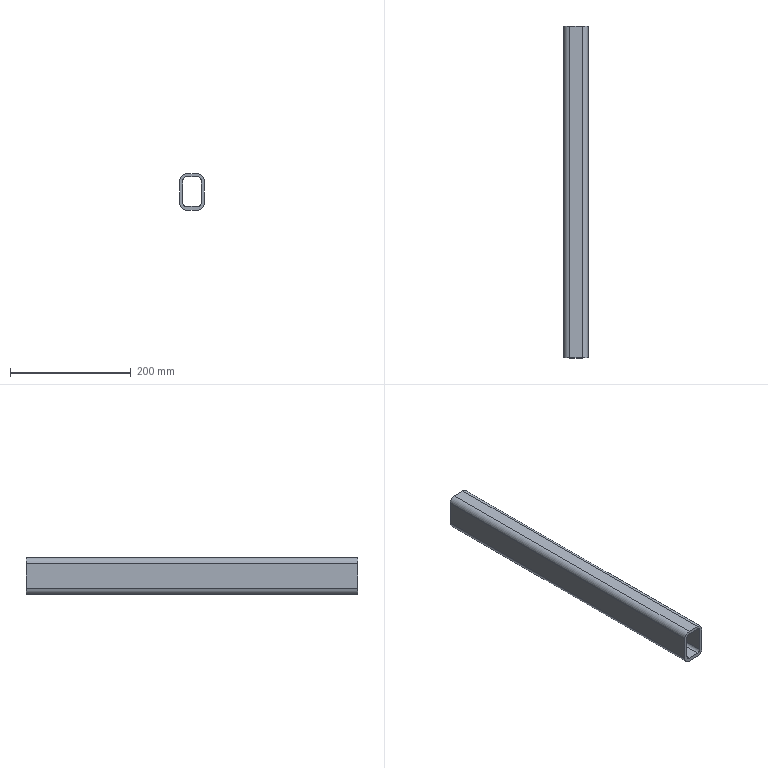Part | STEP file | frame longitudinal beam--000.001--20240926 | 1 solid | 18 faces | box 40 x 550 x 60 mm | volume 476091 mm3 | plane 10 | cylinder 8 | commonest cylinder face diameters 10 x4 20 x4
STEP:
#1=CARTESIAN_POINT('',(0.,0.,0.));
#2=DIRECTION('',(0.,0.,1.));
#3=DIRECTION('',(1.,0.,0.));
#4=AXIS2_PLACEMENT_3D('',#1,#2,#3);
#5=CARTESIAN_POINT('',(-30.,-840.,50.));
#6=VERTEX_POINT('',#5);
#7=CARTESIAN_POINT('',(-30.,-290.,50.));
#8=VERTEX_POINT('',#7);
#9=CARTESIAN_POINT('',(-30.,490.173,50.));
#10=DIRECTION('',(0.,1.,0.));
#11=VECTOR('',#10,1.);
#12=LINE('',#9,#11);
#13=CARTESIAN_POINT('',(-30.,490.173,40.));
#14=DIRECTION('',(0.,1.,0.));
#15=DIRECTION('',(0.,0.,-1.));
#16=AXIS2_PLACEMENT_3D('',#13,#14,#15);
#17=CYLINDRICAL_SURFACE('',#16,10.);
#18=CARTESIAN_POINT('',(3.142,0.));
#19=DIRECTION('',(0.,1.));
#20=VECTOR('',#19,1.);
#21=LINE('',#18,#20);
#22=(GEOMETRIC_REPRESENTATION_CONTEXT(2)PARAMETRIC_REPRESENTATION_CONTEXT()REPRESENTATION_CONTEXT('',''));
#23=DEFINITIONAL_REPRESENTATION('',(#21),#22);
#24=PCURVE('',#17,#23);
#25=CARTESIAN_POINT('',(-40.,490.173,50.));
#26=DIRECTION('',(0.,0.,-1.));
#27=DIRECTION('',(0.,-1.,0.));
#28=AXIS2_PLACEMENT_3D('',#25,#26,#27);
#29=PLANE('',#28);
#30=CARTESIAN_POINT('',(0.,-10.));
#31=DIRECTION('',(-1.,0.));
#32=VECTOR('',#31,1.);
#33=LINE('',#30,#32);
#34=(GEOMETRIC_REPRESENTATION_CONTEXT(2)PARAMETRIC_REPRESENTATION_CONTEXT()REPRESENTATION_CONTEXT('',''));
#35=DEFINITIONAL_REPRESENTATION('',(#33),#34);
#36=PCURVE('',#29,#35);
#37=SURFACE_CURVE('',#12,(#24,#36),.PCURVE_S1.);
#38=EDGE_CURVE('',#6,#8,#37,.T.);
#39=ORIENTED_EDGE('',*,*,#38,.T.);
#40=CARTESIAN_POINT('',(-40.,-290.,40.));
#41=VERTEX_POINT('',#40);
#42=CARTESIAN_POINT('',(-30.,-290.,40.));
#43=DIRECTION('',(0.,-1.,0.));
#44=DIRECTION('',(0.,0.,1.));
#45=AXIS2_PLACEMENT_3D('',#42,#43,#44);
#46=CIRCLE('',#45,10.);
#47=CARTESIAN_POINT('',(3.142,-780.173));
#48=DIRECTION('',(-1.,0.));
#49=VECTOR('',#48,1.);
#50=LINE('',#47,#49);
#51=(GEOMETRIC_REPRESENTATION_CONTEXT(2)PARAMETRIC_REPRESENTATION_CONTEXT()REPRESENTATION_CONTEXT('',''));
#52=DEFINITIONAL_REPRESENTATION('',(#50),#51);
#53=PCURVE('',#17,#52);
#54=CARTESIAN_POINT('',(-399.25,-290.,20.));
#55=DIRECTION('',(0.,1.,0.));
#56=DIRECTION('',(0.,0.,-1.));
#57=AXIS2_PLACEMENT_3D('',#54,#55,#56);
#58=PLANE('',#57);
#59=CARTESIAN_POINT('',(-30.,-369.25));
#60=CARTESIAN_POINT('',(-30.,-351.929));
#61=CARTESIAN_POINT('',(-15.,-360.59));
#62=CARTESIAN_POINT('',(0.,-369.25));
#63=CARTESIAN_POINT('',(-15.,-377.91));
#64=CARTESIAN_POINT('',(-30.,-386.571));
#65=CARTESIAN_POINT('',(-30.,-369.25));
#66=(BOUNDED_CURVE()B_SPLINE_CURVE(2,(#59,#60,#61,#62,#63,#64,#65),.UNSPECIFIED.,.T.,.F.)B_SPLINE_CURVE_WITH_KNOTS((1,2,2,2,2,1),(-2.094,0.,2.094,4.189,6.283,8.378),.UNSPECIFIED.)CURVE()GEOMETRIC_REPRESENTATION_ITEM()RATIONAL_B_SPLINE_CURVE((1.,0.5,1.,0.5,1.,0.5,1.))REPRESENTATION_ITEM(''));
#67=(GEOMETRIC_REPRESENTATION_CONTEXT(2)PARAMETRIC_REPRESENTATION_CONTEXT()REPRESENTATION_CONTEXT('',''));
#68=DEFINITIONAL_REPRESENTATION('',(#66),#67);
#69=PCURVE('',#58,#68);
#70=SURFACE_CURVE('',#46,(#53,#69),.PCURVE_S1.);
#71=EDGE_CURVE('',#8,#41,#70,.T.);
#72=ORIENTED_EDGE('',*,*,#71,.T.);
#73=CARTESIAN_POINT('',(-40.,-840.,40.));
#74=VERTEX_POINT('',#73);
#75=CARTESIAN_POINT('',(-40.,490.173,40.));
#76=DIRECTION('',(0.,-1.,0.));
#77=VECTOR('',#76,1.);
#78=LINE('',#75,#77);
#79=CARTESIAN_POINT('',(1.571,0.));
#80=DIRECTION('',(0.,-1.));
#81=VECTOR('',#80,1.);
#82=LINE('',#79,#81);
#83=(GEOMETRIC_REPRESENTATION_CONTEXT(2)PARAMETRIC_REPRESENTATION_CONTEXT()REPRESENTATION_CONTEXT('',''));
#84=DEFINITIONAL_REPRESENTATION('',(#82),#83);
#85=PCURVE('',#17,#84);
#86=CARTESIAN_POINT('',(-40.,490.173,10.));
#87=DIRECTION('',(1.,0.,0.));
#88=DIRECTION('',(0.,0.9613,-0.2756));
#89=AXIS2_PLACEMENT_3D('',#86,#87,#88);
#90=PLANE('',#89);
#91=CARTESIAN_POINT('',(-8.269,28.838));
#92=DIRECTION('',(-0.9613,-0.2756));
#93=VECTOR('',#92,1.);
#94=LINE('',#91,#93);
#95=(GEOMETRIC_REPRESENTATION_CONTEXT(2)PARAMETRIC_REPRESENTATION_CONTEXT()REPRESENTATION_CONTEXT('',''));
#96=DEFINITIONAL_REPRESENTATION('',(#94),#95);
#97=PCURVE('',#90,#96);
#98=SURFACE_CURVE('',#78,(#85,#97),.PCURVE_S1.);
#99=EDGE_CURVE('',#41,#74,#98,.T.);
#100=ORIENTED_EDGE('',*,*,#99,.T.);
#101=CARTESIAN_POINT('',(-30.,-840.,40.));
#102=DIRECTION('',(0.,-1.,0.));
#103=DIRECTION('',(0.,0.,1.));
#104=AXIS2_PLACEMENT_3D('',#101,#102,#103);
#105=CIRCLE('',#104,10.);
#106=CARTESIAN_POINT('',(3.142,-1330.173));
#107=DIRECTION('',(-1.,0.));
#108=VECTOR('',#107,1.);
#109=LINE('',#106,#108);
#110=(GEOMETRIC_REPRESENTATION_CONTEXT(2)PARAMETRIC_REPRESENTATION_CONTEXT()REPRESENTATION_CONTEXT('',''));
#111=DEFINITIONAL_REPRESENTATION('',(#109),#110);
#112=PCURVE('',#17,#111);
#113=CARTESIAN_POINT('',(-40.,-840.,-10.));
#114=DIRECTION('',(0.,1.,0.));
#115=DIRECTION('',(0.,0.,-1.));
#116=AXIS2_PLACEMENT_3D('',#113,#114,#115);
#117=PLANE('',#116);
#118=CARTESIAN_POINT('',(-60.,-10.));
#119=CARTESIAN_POINT('',(-60.,7.321));
#120=CARTESIAN_POINT('',(-45.,-1.34));
#121=CARTESIAN_POINT('',(-30.,-10.));
#122=CARTESIAN_POINT('',(-45.,-18.66));
#123=CARTESIAN_POINT('',(-60.,-27.321));
#124=CARTESIAN_POINT('',(-60.,-10.));
#125=(BOUNDED_CURVE()B_SPLINE_CURVE(2,(#118,#119,#120,#121,#122,#123,#124),.UNSPECIFIED.,.T.,.F.)B_SPLINE_CURVE_WITH_KNOTS((1,2,2,2,2,1),(-2.094,0.,2.094,4.189,6.283,8.378),.UNSPECIFIED.)CURVE()GEOMETRIC_REPRESENTATION_ITEM()RATIONAL_B_SPLINE_CURVE((1.,0.5,1.,0.5,1.,0.5,1.))REPRESENTATION_ITEM(''));
#126=(GEOMETRIC_REPRESENTATION_CONTEXT(2)PARAMETRIC_REPRESENTATION_CONTEXT()REPRESENTATION_CONTEXT('',''));
#127=DEFINITIONAL_REPRESENTATION('',(#125),#126);
#128=PCURVE('',#117,#127);
#129=SURFACE_CURVE('',#105,(#112,#128),.PCURVE_S1.);
#130=EDGE_CURVE('',#6,#74,#129,.T.);
#131=ORIENTED_EDGE('',*,*,#130,.F.);
#132=EDGE_LOOP('',(#39,#72,#100,#131));
#133=FACE_BOUND('',#132,.T.);
#134=ADVANCED_FACE('',(#133),#17,.T.);
#135=CARTESIAN_POINT('',(-40.,-840.,0.));
#136=VERTEX_POINT('',#135);
#137=CARTESIAN_POINT('',(-40.,-290.,0.));
#138=VERTEX_POINT('',#137);
#139=CARTESIAN_POINT('',(-40.,1110.173,0.));
#140=DIRECTION('',(0.,1.,0.));
#141=VECTOR('',#140,1.);
#142=LINE('',#139,#141);
#143=CARTESIAN_POINT('',(-30.,1110.173,0.));
#144=DIRECTION('',(0.,1.,0.));
#145=DIRECTION('',(0.,0.,-1.));
#146=AXIS2_PLACEMENT_3D('',#143,#144,#145);
#147=CYLINDRICAL_SURFACE('',#146,10.);
#148=CARTESIAN_POINT('',(1.571,0.));
#149=DIRECTION('',(0.,1.));
#150=VECTOR('',#149,1.);
#151=LINE('',#148,#150);
#152=(GEOMETRIC_REPRESENTATION_CONTEXT(2)PARAMETRIC_REPRESENTATION_CONTEXT()REPRESENTATION_CONTEXT('',''));
#153=DEFINITIONAL_REPRESENTATION('',(#151),#152);
#154=PCURVE('',#147,#153);
#155=CARTESIAN_POINT('',(598.739,161.283));
#156=DIRECTION('',(0.9613,0.2756));
#157=VECTOR('',#156,1.);
#158=LINE('',#155,#157);
#159=(GEOMETRIC_REPRESENTATION_CONTEXT(2)PARAMETRIC_REPRESENTATION_CONTEXT()REPRESENTATION_CONTEXT('',''));
#160=DEFINITIONAL_REPRESENTATION('',(#158),#159);
#161=PCURVE('',#90,#160);
#162=SURFACE_CURVE('',#142,(#154,#161),.PCURVE_S1.);
#163=EDGE_CURVE('',#136,#138,#162,.T.);
#164=ORIENTED_EDGE('',*,*,#163,.T.);
#165=CARTESIAN_POINT('',(-30.,-290.,-10.));
#166=VERTEX_POINT('',#165);
#167=CARTESIAN_POINT('',(-30.,-290.,0.));
#168=DIRECTION('',(0.,-1.,0.));
#169=DIRECTION('',(0.,0.,1.));
#170=AXIS2_PLACEMENT_3D('',#167,#168,#169);
#171=CIRCLE('',#170,10.);
#172=CARTESIAN_POINT('',(3.142,-1400.173));
#173=DIRECTION('',(-1.,0.));
#174=VECTOR('',#173,1.);
#175=LINE('',#172,#174);
#176=(GEOMETRIC_REPRESENTATION_CONTEXT(2)PARAMETRIC_REPRESENTATION_CONTEXT()REPRESENTATION_CONTEXT('',''));
#177=DEFINITIONAL_REPRESENTATION('',(#175),#176);
#178=PCURVE('',#147,#177);
#179=CARTESIAN_POINT('',(10.,-369.25));
#180=CARTESIAN_POINT('',(10.,-351.929));
#181=CARTESIAN_POINT('',(25.,-360.59));
#182=CARTESIAN_POINT('',(40.,-369.25));
#183=CARTESIAN_POINT('',(25.,-377.91));
#184=CARTESIAN_POINT('',(10.,-386.571));
#185=CARTESIAN_POINT('',(10.,-369.25));
#186=(BOUNDED_CURVE()B_SPLINE_CURVE(2,(#179,#180,#181,#182,#183,#184,#185),.UNSPECIFIED.,.T.,.F.)B_SPLINE_CURVE_WITH_KNOTS((1,2,2,2,2,1),(-2.094,0.,2.094,4.189,6.283,8.378),.UNSPECIFIED.)CURVE()GEOMETRIC_REPRESENTATION_ITEM()RATIONAL_B_SPLINE_CURVE((1.,0.5,1.,0.5,1.,0.5,1.))REPRESENTATION_ITEM(''));
#187=(GEOMETRIC_REPRESENTATION_CONTEXT(2)PARAMETRIC_REPRESENTATION_CONTEXT()REPRESENTATION_CONTEXT('',''));
#188=DEFINITIONAL_REPRESENTATION('',(#186),#187);
#189=PCURVE('',#58,#188);
#190=SURFACE_CURVE('',#171,(#178,#189),.PCURVE_S1.);
#191=EDGE_CURVE('',#138,#166,#190,.T.);
#192=ORIENTED_EDGE('',*,*,#191,.T.);
#193=CARTESIAN_POINT('',(-30.,-840.,-10.));
#194=VERTEX_POINT('',#193);
#195=CARTESIAN_POINT('',(-30.,1110.173,-10.));
#196=DIRECTION('',(0.,-1.,0.));
#197=VECTOR('',#196,1.);
#198=LINE('',#195,#197);
#199=CARTESIAN_POINT('',(0.,0.));
#200=DIRECTION('',(0.,-1.));
#201=VECTOR('',#200,1.);
#202=LINE('',#199,#201);
#203=(GEOMETRIC_REPRESENTATION_CONTEXT(2)PARAMETRIC_REPRESENTATION_CONTEXT()REPRESENTATION_CONTEXT('',''));
#204=DEFINITIONAL_REPRESENTATION('',(#202),#203);
#205=PCURVE('',#147,#204);
#206=CARTESIAN_POINT('',(0.,1110.173,-10.));
#207=DIRECTION('',(0.,0.,1.));
#208=DIRECTION('',(0.,1.,0.));
#209=AXIS2_PLACEMENT_3D('',#206,#207,#208);
#210=PLANE('',#209);
#211=CARTESIAN_POINT('',(0.,30.));
#212=DIRECTION('',(-1.,0.));
#213=VECTOR('',#212,1.);
#214=LINE('',#211,#213);
#215=(GEOMETRIC_REPRESENTATION_CONTEXT(2)PARAMETRIC_REPRESENTATION_CONTEXT()REPRESENTATION_CONTEXT('',''));
#216=DEFINITIONAL_REPRESENTATION('',(#214),#215);
#217=PCURVE('',#210,#216);
#218=SURFACE_CURVE('',#198,(#205,#217),.PCURVE_S1.);
#219=EDGE_CURVE('',#166,#194,#218,.T.);
#220=ORIENTED_EDGE('',*,*,#219,.T.);
#221=CARTESIAN_POINT('',(-30.,-840.,0.));
#222=DIRECTION('',(0.,-1.,0.));
#223=DIRECTION('',(0.,0.,1.));
#224=AXIS2_PLACEMENT_3D('',#221,#222,#223);
#225=CIRCLE('',#224,10.);
#226=CARTESIAN_POINT('',(3.142,-1950.173));
#227=DIRECTION('',(-1.,0.));
#228=VECTOR('',#227,1.);
#229=LINE('',#226,#228);
#230=(GEOMETRIC_REPRESENTATION_CONTEXT(2)PARAMETRIC_REPRESENTATION_CONTEXT()REPRESENTATION_CONTEXT('',''));
#231=DEFINITIONAL_REPRESENTATION('',(#229),#230);
#232=PCURVE('',#147,#231);
#233=CARTESIAN_POINT('',(-20.,-10.));
#234=CARTESIAN_POINT('',(-20.,7.321));
#235=CARTESIAN_POINT('',(-5.,-1.34));
#236=CARTESIAN_POINT('',(10.,-10.));
#237=CARTESIAN_POINT('',(-5.,-18.66));
#238=CARTESIAN_POINT('',(-20.,-27.321));
#239=CARTESIAN_POINT('',(-20.,-10.));
#240=(BOUNDED_CURVE()B_SPLINE_CURVE(2,(#233,#234,#235,#236,#237,#238,#239),.UNSPECIFIED.,.T.,.F.)B_SPLINE_CURVE_WITH_KNOTS((1,2,2,2,2,1),(-2.094,0.,2.094,4.189,6.283,8.378),.UNSPECIFIED.)CURVE()GEOMETRIC_REPRESENTATION_ITEM()RATIONAL_B_SPLINE_CURVE((1.,0.5,1.,0.5,1.,0.5,1.))REPRESENTATION_ITEM(''));
#241=(GEOMETRIC_REPRESENTATION_CONTEXT(2)PARAMETRIC_REPRESENTATION_CONTEXT()REPRESENTATION_CONTEXT('',''));
#242=DEFINITIONAL_REPRESENTATION('',(#240),#241);
#243=PCURVE('',#117,#242);
#244=SURFACE_CURVE('',#225,(#232,#243),.PCURVE_S1.);
#245=EDGE_CURVE('',#136,#194,#244,.T.);
#246=ORIENTED_EDGE('',*,*,#245,.F.);
#247=EDGE_LOOP('',(#164,#192,#220,#246));
#248=FACE_BOUND('',#247,.T.);
#249=ADVANCED_FACE('',(#248),#147,.T.);
#250=CARTESIAN_POINT('',(-40.,-290.,10.));
#251=DIRECTION('',(0.,0.,1.));
#252=VECTOR('',#251,1.);
#253=LINE('',#250,#252);
#254=CARTESIAN_POINT('',(-749.951,-215.045));
#255=DIRECTION('',(-0.2756,0.9613));
#256=VECTOR('',#255,1.);
#257=LINE('',#254,#256);
#258=(GEOMETRIC_REPRESENTATION_CONTEXT(2)PARAMETRIC_REPRESENTATION_CONTEXT()REPRESENTATION_CONTEXT('',''));
#259=DEFINITIONAL_REPRESENTATION('',(#257),#258);
#260=PCURVE('',#90,#259);
#261=CARTESIAN_POINT('',(10.,-359.25));
#262=DIRECTION('',(-1.,0.));
#263=VECTOR('',#262,1.);
#264=LINE('',#261,#263);
#265=(GEOMETRIC_REPRESENTATION_CONTEXT(2)PARAMETRIC_REPRESENTATION_CONTEXT()REPRESENTATION_CONTEXT('',''));
#266=DEFINITIONAL_REPRESENTATION('',(#264),#265);
#267=PCURVE('',#58,#266);
#268=SURFACE_CURVE('',#253,(#260,#267),.PCURVE_S1.);
#269=EDGE_CURVE('',#138,#41,#268,.T.);
#270=ORIENTED_EDGE('',*,*,#269,.F.);
#271=ORIENTED_EDGE('',*,*,#163,.F.);
#272=CARTESIAN_POINT('',(-40.,-840.,10.));
#273=DIRECTION('',(0.,0.,1.));
#274=VECTOR('',#273,1.);
#275=LINE('',#272,#274);
#276=CARTESIAN_POINT('',(-1278.645,-366.645));
#277=DIRECTION('',(-0.2756,0.9613));
#278=VECTOR('',#277,1.);
#279=LINE('',#276,#278);
#280=(GEOMETRIC_REPRESENTATION_CONTEXT(2)PARAMETRIC_REPRESENTATION_CONTEXT()REPRESENTATION_CONTEXT('',''));
#281=DEFINITIONAL_REPRESENTATION('',(#279),#280);
#282=PCURVE('',#90,#281);
#283=CARTESIAN_POINT('',(-20.,0.));
#284=DIRECTION('',(-1.,0.));
#285=VECTOR('',#284,1.);
#286=LINE('',#283,#285);
#287=(GEOMETRIC_REPRESENTATION_CONTEXT(2)PARAMETRIC_REPRESENTATION_CONTEXT()REPRESENTATION_CONTEXT('',''));
#288=DEFINITIONAL_REPRESENTATION('',(#286),#287);
#289=PCURVE('',#117,#288);
#290=SURFACE_CURVE('',#275,(#282,#289),.PCURVE_S1.);
#291=EDGE_CURVE('',#136,#74,#290,.T.);
#292=ORIENTED_EDGE('',*,*,#291,.T.);
#293=ORIENTED_EDGE('',*,*,#99,.F.);
#294=EDGE_LOOP('',(#270,#271,#292,#293));
#295=FACE_BOUND('',#294,.T.);
#296=ADVANCED_FACE('',(#295),#90,.F.);
#297=CARTESIAN_POINT('',(-10.,-840.,-10.));
#298=VERTEX_POINT('',#297);
#299=CARTESIAN_POINT('',(-10.,-290.,-10.));
#300=VERTEX_POINT('',#299);
#301=CARTESIAN_POINT('',(-10.,490.173,-10.));
#302=DIRECTION('',(0.,1.,0.));
#303=VECTOR('',#302,1.);
#304=LINE('',#301,#303);
#305=CARTESIAN_POINT('',(-10.,490.173,0.));
#306=DIRECTION('',(0.,1.,0.));
#307=DIRECTION('',(0.,0.,-1.));
#308=AXIS2_PLACEMENT_3D('',#305,#306,#307);
#309=CYLINDRICAL_SURFACE('',#308,10.);
#310=CARTESIAN_POINT('',(6.283,0.));
#311=DIRECTION('',(0.,1.));
#312=VECTOR('',#311,1.);
#313=LINE('',#310,#312);
#314=(GEOMETRIC_REPRESENTATION_CONTEXT(2)PARAMETRIC_REPRESENTATION_CONTEXT()REPRESENTATION_CONTEXT('',''));
#315=DEFINITIONAL_REPRESENTATION('',(#313),#314);
#316=PCURVE('',#309,#315);
#317=CARTESIAN_POINT('',(-620.,10.));
#318=DIRECTION('',(1.,0.));
#319=VECTOR('',#318,1.);
#320=LINE('',#317,#319);
#321=(GEOMETRIC_REPRESENTATION_CONTEXT(2)PARAMETRIC_REPRESENTATION_CONTEXT()REPRESENTATION_CONTEXT('',''));
#322=DEFINITIONAL_REPRESENTATION('',(#320),#321);
#323=PCURVE('',#210,#322);
#324=SURFACE_CURVE('',#304,(#316,#323),.PCURVE_S1.);
#325=EDGE_CURVE('',#298,#300,#324,.T.);
#326=ORIENTED_EDGE('',*,*,#325,.T.);
#327=CARTESIAN_POINT('',(0.,-290.,0.));
#328=VERTEX_POINT('',#327);
#329=CARTESIAN_POINT('',(-10.,-290.,0.));
#330=DIRECTION('',(0.,-1.,0.));
#331=DIRECTION('',(0.,0.,1.));
#332=AXIS2_PLACEMENT_3D('',#329,#330,#331);
#333=CIRCLE('',#332,10.);
#334=CARTESIAN_POINT('',(9.425,-780.173));
#335=DIRECTION('',(-1.,0.));
#336=VECTOR('',#335,1.);
#337=LINE('',#334,#336);
#338=(GEOMETRIC_REPRESENTATION_CONTEXT(2)PARAMETRIC_REPRESENTATION_CONTEXT()REPRESENTATION_CONTEXT('',''));
#339=DEFINITIONAL_REPRESENTATION('',(#337),#338);
#340=PCURVE('',#309,#339);
#341=CARTESIAN_POINT('',(10.,-389.25));
#342=CARTESIAN_POINT('',(10.,-371.929));
#343=CARTESIAN_POINT('',(25.,-380.59));
#344=CARTESIAN_POINT('',(40.,-389.25));
#345=CARTESIAN_POINT('',(25.,-397.91));
#346=CARTESIAN_POINT('',(10.,-406.571));
#347=CARTESIAN_POINT('',(10.,-389.25));
#348=(BOUNDED_CURVE()B_SPLINE_CURVE(2,(#341,#342,#343,#344,#345,#346,#347),.UNSPECIFIED.,.T.,.F.)B_SPLINE_CURVE_WITH_KNOTS((1,2,2,2,2,1),(-2.094,0.,2.094,4.189,6.283,8.378),.UNSPECIFIED.)CURVE()GEOMETRIC_REPRESENTATION_ITEM()RATIONAL_B_SPLINE_CURVE((1.,0.5,1.,0.5,1.,0.5,1.))REPRESENTATION_ITEM(''));
#349=(GEOMETRIC_REPRESENTATION_CONTEXT(2)PARAMETRIC_REPRESENTATION_CONTEXT()REPRESENTATION_CONTEXT('',''));
#350=DEFINITIONAL_REPRESENTATION('',(#348),#349);
#351=PCURVE('',#58,#350);
#352=SURFACE_CURVE('',#333,(#340,#351),.PCURVE_S1.);
#353=EDGE_CURVE('',#300,#328,#352,.T.);
#354=ORIENTED_EDGE('',*,*,#353,.T.);
#355=CARTESIAN_POINT('',(0.,-840.,0.));
#356=VERTEX_POINT('',#355);
#357=CARTESIAN_POINT('',(0.,490.173,0.));
#358=DIRECTION('',(0.,-1.,0.));
#359=VECTOR('',#358,1.);
#360=LINE('',#357,#359);
#361=CARTESIAN_POINT('',(4.712,0.));
#362=DIRECTION('',(0.,-1.));
#363=VECTOR('',#362,1.);
#364=LINE('',#361,#363);
#365=(GEOMETRIC_REPRESENTATION_CONTEXT(2)PARAMETRIC_REPRESENTATION_CONTEXT()REPRESENTATION_CONTEXT('',''));
#366=DEFINITIONAL_REPRESENTATION('',(#364),#365);
#367=PCURVE('',#309,#366);
#368=CARTESIAN_POINT('',(0.,490.173,50.));
#369=DIRECTION('',(-1.,0.,0.));
#370=DIRECTION('',(0.,-0.9613,0.2756));
#371=AXIS2_PLACEMENT_3D('',#368,#369,#370);
#372=PLANE('',#371);
#373=CARTESIAN_POINT('',(-13.782,-48.063));
#374=DIRECTION('',(0.9613,-0.2756));
#375=VECTOR('',#374,1.);
#376=LINE('',#373,#375);
#377=(GEOMETRIC_REPRESENTATION_CONTEXT(2)PARAMETRIC_REPRESENTATION_CONTEXT()REPRESENTATION_CONTEXT('',''));
#378=DEFINITIONAL_REPRESENTATION('',(#376),#377);
#379=PCURVE('',#372,#378);
#380=SURFACE_CURVE('',#360,(#367,#379),.PCURVE_S1.);
#381=EDGE_CURVE('',#328,#356,#380,.T.);
#382=ORIENTED_EDGE('',*,*,#381,.T.);
#383=CARTESIAN_POINT('',(-10.,-840.,0.));
#384=DIRECTION('',(0.,1.,0.));
#385=DIRECTION('',(0.,0.,1.));
#386=AXIS2_PLACEMENT_3D('',#383,#384,#385);
#387=CIRCLE('',#386,10.);
#388=CARTESIAN_POINT('',(3.142,-1330.173));
#389=DIRECTION('',(1.,0.));
#390=VECTOR('',#389,1.);
#391=LINE('',#388,#390);
#392=(GEOMETRIC_REPRESENTATION_CONTEXT(2)PARAMETRIC_REPRESENTATION_CONTEXT()REPRESENTATION_CONTEXT('',''));
#393=DEFINITIONAL_REPRESENTATION('',(#391),#392);
#394=PCURVE('',#309,#393);
#395=CARTESIAN_POINT('',(-10.,-30.));
#396=DIRECTION('',(-1.,0.));
#397=AXIS2_PLACEMENT_2D('',#395,#396);
#398=CIRCLE('',#397,10.);
#399=(GEOMETRIC_REPRESENTATION_CONTEXT(2)PARAMETRIC_REPRESENTATION_CONTEXT()REPRESENTATION_CONTEXT('',''));
#400=DEFINITIONAL_REPRESENTATION('',(#398),#399);
#401=PCURVE('',#117,#400);
#402=SURFACE_CURVE('',#387,(#394,#401),.PCURVE_S1.);
#403=EDGE_CURVE('',#356,#298,#402,.T.);
#404=ORIENTED_EDGE('',*,*,#403,.T.);
#405=EDGE_LOOP('',(#326,#354,#382,#404));
#406=FACE_BOUND('',#405,.T.);
#407=ADVANCED_FACE('',(#406),#309,.T.);
#408=CARTESIAN_POINT('',(0.,-290.,-10.));
#409=DIRECTION('',(-1.,0.,0.));
#410=VECTOR('',#409,1.);
#411=LINE('',#408,#410);
#412=CARTESIAN_POINT('',(-1400.173,0.));
#413=DIRECTION('',(0.,1.));
#414=VECTOR('',#413,1.);
#415=LINE('',#412,#414);
#416=(GEOMETRIC_REPRESENTATION_CONTEXT(2)PARAMETRIC_REPRESENTATION_CONTEXT()REPRESENTATION_CONTEXT('',''));
#417=DEFINITIONAL_REPRESENTATION('',(#415),#416);
#418=PCURVE('',#210,#417);
#419=CARTESIAN_POINT('',(30.,-399.25));
#420=DIRECTION('',(0.,1.));
#421=VECTOR('',#420,1.);
#422=LINE('',#419,#421);
#423=(GEOMETRIC_REPRESENTATION_CONTEXT(2)PARAMETRIC_REPRESENTATION_CONTEXT()REPRESENTATION_CONTEXT('',''));
#424=DEFINITIONAL_REPRESENTATION('',(#422),#423);
#425=PCURVE('',#58,#424);
#426=SURFACE_CURVE('',#411,(#418,#425),.PCURVE_S1.);
#427=EDGE_CURVE('',#300,#166,#426,.T.);
#428=ORIENTED_EDGE('',*,*,#427,.F.);
#429=ORIENTED_EDGE('',*,*,#325,.F.);
#430=CARTESIAN_POINT('',(-40.,-840.,-10.));
#431=DIRECTION('',(1.,0.,0.));
#432=VECTOR('',#431,1.);
#433=LINE('',#430,#432);
#434=CARTESIAN_POINT('',(-1950.173,40.));
#435=DIRECTION('',(0.,-1.));
#436=VECTOR('',#435,1.);
#437=LINE('',#434,#436);
#438=(GEOMETRIC_REPRESENTATION_CONTEXT(2)PARAMETRIC_REPRESENTATION_CONTEXT()REPRESENTATION_CONTEXT('',''));
#439=DEFINITIONAL_REPRESENTATION('',(#437),#438);
#440=PCURVE('',#210,#439);
#441=CARTESIAN_POINT('',(0.,0.));
#442=DIRECTION('',(0.,-1.));
#443=VECTOR('',#442,1.);
#444=LINE('',#441,#443);
#445=(GEOMETRIC_REPRESENTATION_CONTEXT(2)PARAMETRIC_REPRESENTATION_CONTEXT()REPRESENTATION_CONTEXT('',''));
#446=DEFINITIONAL_REPRESENTATION('',(#444),#445);
#447=PCURVE('',#117,#446);
#448=SURFACE_CURVE('',#433,(#440,#447),.PCURVE_S1.);
#449=EDGE_CURVE('',#194,#298,#448,.T.);
#450=ORIENTED_EDGE('',*,*,#449,.F.);
#451=ORIENTED_EDGE('',*,*,#219,.F.);
#452=EDGE_LOOP('',(#428,#429,#450,#451));
#453=FACE_BOUND('',#452,.T.);
#454=ADVANCED_FACE('',(#453),#210,.F.);
#455=CARTESIAN_POINT('',(0.,-840.,40.));
#456=VERTEX_POINT('',#455);
#457=CARTESIAN_POINT('',(0.,-290.,40.));
#458=VERTEX_POINT('',#457);
#459=CARTESIAN_POINT('',(0.,490.173,40.));
#460=DIRECTION('',(0.,1.,0.));
#461=VECTOR('',#460,1.);
#462=LINE('',#459,#461);
#463=CARTESIAN_POINT('',(-10.,490.173,40.));
#464=DIRECTION('',(0.,1.,0.));
#465=DIRECTION('',(0.,0.,-1.));
#466=AXIS2_PLACEMENT_3D('',#463,#464,#465);
#467=CYLINDRICAL_SURFACE('',#466,10.);
#468=CARTESIAN_POINT('',(4.712,0.));
#469=DIRECTION('',(0.,1.));
#470=VECTOR('',#469,1.);
#471=LINE('',#468,#470);
#472=(GEOMETRIC_REPRESENTATION_CONTEXT(2)PARAMETRIC_REPRESENTATION_CONTEXT()REPRESENTATION_CONTEXT('',''));
#473=DEFINITIONAL_REPRESENTATION('',(#471),#472);
#474=PCURVE('',#467,#473);
#475=CARTESIAN_POINT('',(-2.756,-9.613));
#476=DIRECTION('',(-0.9613,0.2756));
#477=VECTOR('',#476,1.);
#478=LINE('',#475,#477);
#479=(GEOMETRIC_REPRESENTATION_CONTEXT(2)PARAMETRIC_REPRESENTATION_CONTEXT()REPRESENTATION_CONTEXT('',''));
#480=DEFINITIONAL_REPRESENTATION('',(#478),#479);
#481=PCURVE('',#372,#480);
#482=SURFACE_CURVE('',#462,(#474,#481),.PCURVE_S1.);
#483=EDGE_CURVE('',#456,#458,#482,.T.);
#484=ORIENTED_EDGE('',*,*,#483,.T.);
#485=CARTESIAN_POINT('',(-10.,-290.,50.));
#486=VERTEX_POINT('',#485);
#487=CARTESIAN_POINT('',(-10.,-290.,40.));
#488=DIRECTION('',(0.,-1.,0.));
#489=DIRECTION('',(0.,0.,1.));
#490=AXIS2_PLACEMENT_3D('',#487,#488,#489);
#491=CIRCLE('',#490,10.);
#492=CARTESIAN_POINT('',(9.425,-780.173));
#493=DIRECTION('',(-1.,0.));
#494=VECTOR('',#493,1.);
#495=LINE('',#492,#494);
#496=(GEOMETRIC_REPRESENTATION_CONTEXT(2)PARAMETRIC_REPRESENTATION_CONTEXT()REPRESENTATION_CONTEXT('',''));
#497=DEFINITIONAL_REPRESENTATION('',(#495),#496);
#498=PCURVE('',#467,#497);
#499=CARTESIAN_POINT('',(-30.,-389.25));
#500=CARTESIAN_POINT('',(-30.,-371.929));
#501=CARTESIAN_POINT('',(-15.,-380.59));
#502=CARTESIAN_POINT('',(0.,-389.25));
#503=CARTESIAN_POINT('',(-15.,-397.91));
#504=CARTESIAN_POINT('',(-30.,-406.571));
#505=CARTESIAN_POINT('',(-30.,-389.25));
#506=(BOUNDED_CURVE()B_SPLINE_CURVE(2,(#499,#500,#501,#502,#503,#504,#505),.UNSPECIFIED.,.T.,.F.)B_SPLINE_CURVE_WITH_KNOTS((1,2,2,2,2,1),(-2.094,0.,2.094,4.189,6.283,8.378),.UNSPECIFIED.)CURVE()GEOMETRIC_REPRESENTATION_ITEM()RATIONAL_B_SPLINE_CURVE((1.,0.5,1.,0.5,1.,0.5,1.))REPRESENTATION_ITEM(''));
#507=(GEOMETRIC_REPRESENTATION_CONTEXT(2)PARAMETRIC_REPRESENTATION_CONTEXT()REPRESENTATION_CONTEXT('',''));
#508=DEFINITIONAL_REPRESENTATION('',(#506),#507);
#509=PCURVE('',#58,#508);
#510=SURFACE_CURVE('',#491,(#498,#509),.PCURVE_S1.);
#511=EDGE_CURVE('',#458,#486,#510,.T.);
#512=ORIENTED_EDGE('',*,*,#511,.T.);
#513=CARTESIAN_POINT('',(-10.,-840.,50.));
#514=VERTEX_POINT('',#513);
#515=CARTESIAN_POINT('',(-10.,490.173,50.));
#516=DIRECTION('',(0.,-1.,0.));
#517=VECTOR('',#516,1.);
#518=LINE('',#515,#517);
#519=CARTESIAN_POINT('',(3.142,0.));
#520=DIRECTION('',(0.,-1.));
#521=VECTOR('',#520,1.);
#522=LINE('',#519,#521);
#523=(GEOMETRIC_REPRESENTATION_CONTEXT(2)PARAMETRIC_REPRESENTATION_CONTEXT()REPRESENTATION_CONTEXT('',''));
#524=DEFINITIONAL_REPRESENTATION('',(#522),#523);
#525=PCURVE('',#467,#524);
#526=CARTESIAN_POINT('',(0.,-30.));
#527=DIRECTION('',(1.,0.));
#528=VECTOR('',#527,1.);
#529=LINE('',#526,#528);
#530=(GEOMETRIC_REPRESENTATION_CONTEXT(2)PARAMETRIC_REPRESENTATION_CONTEXT()REPRESENTATION_CONTEXT('',''));
#531=DEFINITIONAL_REPRESENTATION('',(#529),#530);
#532=PCURVE('',#29,#531);
#533=SURFACE_CURVE('',#518,(#525,#532),.PCURVE_S1.);
#534=EDGE_CURVE('',#486,#514,#533,.T.);
#535=ORIENTED_EDGE('',*,*,#534,.T.);
#536=CARTESIAN_POINT('',(-10.,-840.,40.));
#537=DIRECTION('',(0.,-1.,0.));
#538=DIRECTION('',(0.,0.,1.));
#539=AXIS2_PLACEMENT_3D('',#536,#537,#538);
#540=CIRCLE('',#539,10.);
#541=CARTESIAN_POINT('',(9.425,-1330.173));
#542=DIRECTION('',(-1.,0.));
#543=VECTOR('',#542,1.);
#544=LINE('',#541,#543);
#545=(GEOMETRIC_REPRESENTATION_CONTEXT(2)PARAMETRIC_REPRESENTATION_CONTEXT()REPRESENTATION_CONTEXT('',''));
#546=DEFINITIONAL_REPRESENTATION('',(#544),#545);
#547=PCURVE('',#467,#546);
#548=CARTESIAN_POINT('',(-60.,-30.));
#549=CARTESIAN_POINT('',(-60.,-12.679));
#550=CARTESIAN_POINT('',(-45.,-21.34));
#551=CARTESIAN_POINT('',(-30.,-30.));
#552=CARTESIAN_POINT('',(-45.,-38.66));
#553=CARTESIAN_POINT('',(-60.,-47.321));
#554=CARTESIAN_POINT('',(-60.,-30.));
#555=(BOUNDED_CURVE()B_SPLINE_CURVE(2,(#548,#549,#550,#551,#552,#553,#554),.UNSPECIFIED.,.T.,.F.)B_SPLINE_CURVE_WITH_KNOTS((1,2,2,2,2,1),(-2.094,0.,2.094,4.189,6.283,8.378),.UNSPECIFIED.)CURVE()GEOMETRIC_REPRESENTATION_ITEM()RATIONAL_B_SPLINE_CURVE((1.,0.5,1.,0.5,1.,0.5,1.))REPRESENTATION_ITEM(''));
#556=(GEOMETRIC_REPRESENTATION_CONTEXT(2)PARAMETRIC_REPRESENTATION_CONTEXT()REPRESENTATION_CONTEXT('',''));
#557=DEFINITIONAL_REPRESENTATION('',(#555),#556);
#558=PCURVE('',#117,#557);
#559=SURFACE_CURVE('',#540,(#547,#558),.PCURVE_S1.);
#560=EDGE_CURVE('',#456,#514,#559,.T.);
#561=ORIENTED_EDGE('',*,*,#560,.F.);
#562=EDGE_LOOP('',(#484,#512,#535,#561));
#563=FACE_BOUND('',#562,.T.);
#564=ADVANCED_FACE('',(#563),#467,.T.);
#565=CARTESIAN_POINT('',(0.,-290.,50.));
#566=DIRECTION('',(0.,0.,-1.));
#567=VECTOR('',#566,1.);
#568=LINE('',#565,#567);
#569=CARTESIAN_POINT('',(749.951,-215.045));
#570=DIRECTION('',(-0.2756,-0.9613));
#571=VECTOR('',#570,1.);
#572=LINE('',#569,#571);
#573=(GEOMETRIC_REPRESENTATION_CONTEXT(2)PARAMETRIC_REPRESENTATION_CONTEXT()REPRESENTATION_CONTEXT('',''));
#574=DEFINITIONAL_REPRESENTATION('',(#572),#573);
#575=PCURVE('',#372,#574);
#576=CARTESIAN_POINT('',(-30.,-399.25));
#577=DIRECTION('',(1.,0.));
#578=VECTOR('',#577,1.);
#579=LINE('',#576,#578);
#580=(GEOMETRIC_REPRESENTATION_CONTEXT(2)PARAMETRIC_REPRESENTATION_CONTEXT()REPRESENTATION_CONTEXT('',''));
#581=DEFINITIONAL_REPRESENTATION('',(#579),#580);
#582=PCURVE('',#58,#581);
#583=SURFACE_CURVE('',#568,(#575,#582),.PCURVE_S1.);
#584=EDGE_CURVE('',#458,#328,#583,.T.);
#585=ORIENTED_EDGE('',*,*,#584,.F.);
#586=ORIENTED_EDGE('',*,*,#483,.F.);
#587=CARTESIAN_POINT('',(0.,-840.,50.));
#588=DIRECTION('',(0.,0.,-1.));
#589=VECTOR('',#588,1.);
#590=LINE('',#587,#589);
#591=CARTESIAN_POINT('',(1278.645,-366.645));
#592=DIRECTION('',(-0.2756,-0.9613));
#593=VECTOR('',#592,1.);
#594=LINE('',#591,#593);
#595=(GEOMETRIC_REPRESENTATION_CONTEXT(2)PARAMETRIC_REPRESENTATION_CONTEXT()REPRESENTATION_CONTEXT('',''));
#596=DEFINITIONAL_REPRESENTATION('',(#594),#595);
#597=PCURVE('',#372,#596);
#598=CARTESIAN_POINT('',(-60.,-40.));
#599=DIRECTION('',(1.,0.));
#600=VECTOR('',#599,1.);
#601=LINE('',#598,#600);
#602=(GEOMETRIC_REPRESENTATION_CONTEXT(2)PARAMETRIC_REPRESENTATION_CONTEXT()REPRESENTATION_CONTEXT('',''));
#603=DEFINITIONAL_REPRESENTATION('',(#601),#602);
#604=PCURVE('',#117,#603);
#605=SURFACE_CURVE('',#590,(#597,#604),.PCURVE_S1.);
#606=EDGE_CURVE('',#456,#356,#605,.T.);
#607=ORIENTED_EDGE('',*,*,#606,.T.);
#608=ORIENTED_EDGE('',*,*,#381,.F.);
#609=EDGE_LOOP('',(#585,#586,#607,#608));
#610=FACE_BOUND('',#609,.T.);
#611=ADVANCED_FACE('',(#610),#372,.F.);
#612=CARTESIAN_POINT('',(-40.,-290.,50.));
#613=DIRECTION('',(1.,0.,0.));
#614=VECTOR('',#613,1.);
#615=LINE('',#612,#614);
#616=CARTESIAN_POINT('',(780.173,0.));
#617=DIRECTION('',(0.,-1.));
#618=VECTOR('',#617,1.);
#619=LINE('',#616,#618);
#620=(GEOMETRIC_REPRESENTATION_CONTEXT(2)PARAMETRIC_REPRESENTATION_CONTEXT()REPRESENTATION_CONTEXT('',''));
#621=DEFINITIONAL_REPRESENTATION('',(#619),#620);
#622=PCURVE('',#29,#621);
#623=CARTESIAN_POINT('',(-30.,-359.25));
#624=DIRECTION('',(0.,-1.));
#625=VECTOR('',#624,1.);
#626=LINE('',#623,#625);
#627=(GEOMETRIC_REPRESENTATION_CONTEXT(2)PARAMETRIC_REPRESENTATION_CONTEXT()REPRESENTATION_CONTEXT('',''));
#628=DEFINITIONAL_REPRESENTATION('',(#626),#627);
#629=PCURVE('',#58,#628);
#630=SURFACE_CURVE('',#615,(#622,#629),.PCURVE_S1.);
#631=EDGE_CURVE('',#8,#486,#630,.T.);
#632=ORIENTED_EDGE('',*,*,#631,.F.);
#633=ORIENTED_EDGE('',*,*,#38,.F.);
#634=CARTESIAN_POINT('',(-40.,-840.,50.));
#635=DIRECTION('',(1.,0.,0.));
#636=VECTOR('',#635,1.);
#637=LINE('',#634,#636);
#638=CARTESIAN_POINT('',(1330.173,0.));
#639=DIRECTION('',(0.,-1.));
#640=VECTOR('',#639,1.);
#641=LINE('',#638,#640);
#642=(GEOMETRIC_REPRESENTATION_CONTEXT(2)PARAMETRIC_REPRESENTATION_CONTEXT()REPRESENTATION_CONTEXT('',''));
#643=DEFINITIONAL_REPRESENTATION('',(#641),#642);
#644=PCURVE('',#29,#643);
#645=CARTESIAN_POINT('',(-60.,0.));
#646=DIRECTION('',(0.,-1.));
#647=VECTOR('',#646,1.);
#648=LINE('',#645,#647);
#649=(GEOMETRIC_REPRESENTATION_CONTEXT(2)PARAMETRIC_REPRESENTATION_CONTEXT()REPRESENTATION_CONTEXT('',''));
#650=DEFINITIONAL_REPRESENTATION('',(#648),#649);
#651=PCURVE('',#117,#650);
#652=SURFACE_CURVE('',#637,(#644,#651),.PCURVE_S1.);
#653=EDGE_CURVE('',#6,#514,#652,.T.);
#654=ORIENTED_EDGE('',*,*,#653,.T.);
#655=ORIENTED_EDGE('',*,*,#534,.F.);
#656=EDGE_LOOP('',(#632,#633,#654,#655));
#657=FACE_BOUND('',#656,.T.);
#658=ADVANCED_FACE('',(#657),#29,.F.);
#659=CARTESIAN_POINT('',(-10.,-290.,45.));
#660=VERTEX_POINT('',#659);
#661=CARTESIAN_POINT('',(-10.,-840.,45.));
#662=VERTEX_POINT('',#661);
#663=CARTESIAN_POINT('',(-10.,-1963.827,45.));
#664=DIRECTION('',(0.,-1.,0.));
#665=VECTOR('',#664,1.);
#666=LINE('',#663,#665);
#667=CARTESIAN_POINT('',(-10.,490.173,40.));
#668=DIRECTION('',(0.,-1.,0.));
#669=DIRECTION('',(0.,0.,1.));
#670=AXIS2_PLACEMENT_3D('',#667,#668,#669);
#671=CYLINDRICAL_SURFACE('',#670,5.);
#672=CARTESIAN_POINT('',(6.283,2454.));
#673=DIRECTION('',(0.,1.));
#674=VECTOR('',#673,1.);
#675=LINE('',#672,#674);
#676=(GEOMETRIC_REPRESENTATION_CONTEXT(2)PARAMETRIC_REPRESENTATION_CONTEXT()REPRESENTATION_CONTEXT('',''));
#677=DEFINITIONAL_REPRESENTATION('',(#675),#676);
#678=PCURVE('',#671,#677);
#679=CARTESIAN_POINT('',(-2.,490.173,45.));
#680=DIRECTION('',(0.,0.,1.));
#681=DIRECTION('',(0.,1.,0.));
#682=AXIS2_PLACEMENT_3D('',#679,#680,#681);
#683=PLANE('',#682);
#684=CARTESIAN_POINT('',(-2454.,8.));
#685=DIRECTION('',(-1.,0.));
#686=VECTOR('',#685,1.);
#687=LINE('',#684,#686);
#688=(GEOMETRIC_REPRESENTATION_CONTEXT(2)PARAMETRIC_REPRESENTATION_CONTEXT()REPRESENTATION_CONTEXT('',''));
#689=DEFINITIONAL_REPRESENTATION('',(#687),#688);
#690=PCURVE('',#683,#689);
#691=SURFACE_CURVE('',#666,(#678,#690),.PCURVE_S1.);
#692=EDGE_CURVE('',#660,#662,#691,.T.);
#693=ORIENTED_EDGE('',*,*,#692,.T.);
#694=CARTESIAN_POINT('',(-5.,-840.,40.));
#695=VERTEX_POINT('',#694);
#696=CARTESIAN_POINT('',(-10.,-840.,40.));
#697=DIRECTION('',(0.,-1.,0.));
#698=DIRECTION('',(0.,0.,1.));
#699=AXIS2_PLACEMENT_3D('',#696,#697,#698);
#700=CIRCLE('',#699,5.);
#701=CARTESIAN_POINT('',(0.,1330.173));
#702=DIRECTION('',(1.,0.));
#703=VECTOR('',#702,1.);
#704=LINE('',#701,#703);
#705=(GEOMETRIC_REPRESENTATION_CONTEXT(2)PARAMETRIC_REPRESENTATION_CONTEXT()REPRESENTATION_CONTEXT('',''));
#706=DEFINITIONAL_REPRESENTATION('',(#704),#705);
#707=PCURVE('',#671,#706);
#708=CARTESIAN_POINT('',(-55.,-30.));
#709=CARTESIAN_POINT('',(-55.,-21.34));
#710=CARTESIAN_POINT('',(-47.5,-25.67));
#711=CARTESIAN_POINT('',(-40.,-30.));
#712=CARTESIAN_POINT('',(-47.5,-34.33));
#713=CARTESIAN_POINT('',(-55.,-38.66));
#714=CARTESIAN_POINT('',(-55.,-30.));
#715=(BOUNDED_CURVE()B_SPLINE_CURVE(2,(#708,#709,#710,#711,#712,#713,#714),.UNSPECIFIED.,.T.,.F.)B_SPLINE_CURVE_WITH_KNOTS((1,2,2,2,2,1),(-2.094,0.,2.094,4.189,6.283,8.378),.UNSPECIFIED.)CURVE()GEOMETRIC_REPRESENTATION_ITEM()RATIONAL_B_SPLINE_CURVE((1.,0.5,1.,0.5,1.,0.5,1.))REPRESENTATION_ITEM(''));
#716=(GEOMETRIC_REPRESENTATION_CONTEXT(2)PARAMETRIC_REPRESENTATION_CONTEXT()REPRESENTATION_CONTEXT('',''));
#717=DEFINITIONAL_REPRESENTATION('',(#715),#716);
#718=PCURVE('',#117,#717);
#719=SURFACE_CURVE('',#700,(#707,#718),.PCURVE_S1.);
#720=EDGE_CURVE('',#695,#662,#719,.T.);
#721=ORIENTED_EDGE('',*,*,#720,.F.);
#722=CARTESIAN_POINT('',(-5.,-290.,40.));
#723=VERTEX_POINT('',#722);
#724=CARTESIAN_POINT('',(-5.,-12.827,40.));
#725=DIRECTION('',(0.,1.,0.));
#726=VECTOR('',#725,1.);
#727=LINE('',#724,#726);
#728=CARTESIAN_POINT('',(4.712,503.));
#729=DIRECTION('',(0.,-1.));
#730=VECTOR('',#729,1.);
#731=LINE('',#728,#730);
#732=(GEOMETRIC_REPRESENTATION_CONTEXT(2)PARAMETRIC_REPRESENTATION_CONTEXT()REPRESENTATION_CONTEXT('',''));
#733=DEFINITIONAL_REPRESENTATION('',(#731),#732);
#734=PCURVE('',#671,#733);
#735=CARTESIAN_POINT('',(-5.,490.173,12.));
#736=DIRECTION('',(1.,0.,0.));
#737=DIRECTION('',(0.,0.9613,-0.2756));
#738=AXIS2_PLACEMENT_3D('',#735,#736,#737);
#739=PLANE('',#738);
#740=CARTESIAN_POINT('',(-491.232,-111.73));
#741=DIRECTION('',(0.9613,0.2756));
#742=VECTOR('',#741,1.);
#743=LINE('',#740,#742);
#744=(GEOMETRIC_REPRESENTATION_CONTEXT(2)PARAMETRIC_REPRESENTATION_CONTEXT()REPRESENTATION_CONTEXT('',''));
#745=DEFINITIONAL_REPRESENTATION('',(#743),#744);
#746=PCURVE('',#739,#745);
#747=SURFACE_CURVE('',#727,(#734,#746),.PCURVE_S1.);
#748=EDGE_CURVE('',#695,#723,#747,.T.);
#749=ORIENTED_EDGE('',*,*,#748,.T.);
#750=CARTESIAN_POINT('',(-10.,-290.,40.));
#751=DIRECTION('',(0.,-1.,0.));
#752=DIRECTION('',(0.,0.,1.));
#753=AXIS2_PLACEMENT_3D('',#750,#751,#752);
#754=CIRCLE('',#753,5.);
#755=CARTESIAN_POINT('',(0.,780.173));
#756=DIRECTION('',(1.,0.));
#757=VECTOR('',#756,1.);
#758=LINE('',#755,#757);
#759=(GEOMETRIC_REPRESENTATION_CONTEXT(2)PARAMETRIC_REPRESENTATION_CONTEXT()REPRESENTATION_CONTEXT('',''));
#760=DEFINITIONAL_REPRESENTATION('',(#758),#759);
#761=PCURVE('',#671,#760);
#762=CARTESIAN_POINT('',(-25.,-389.25));
#763=CARTESIAN_POINT('',(-25.,-380.59));
#764=CARTESIAN_POINT('',(-17.5,-384.92));
#765=CARTESIAN_POINT('',(-10.,-389.25));
#766=CARTESIAN_POINT('',(-17.5,-393.58));
#767=CARTESIAN_POINT('',(-25.,-397.91));
#768=CARTESIAN_POINT('',(-25.,-389.25));
#769=(BOUNDED_CURVE()B_SPLINE_CURVE(2,(#762,#763,#764,#765,#766,#767,#768),.UNSPECIFIED.,.T.,.F.)B_SPLINE_CURVE_WITH_KNOTS((1,2,2,2,2,1),(-2.094,0.,2.094,4.189,6.283,8.378),.UNSPECIFIED.)CURVE()GEOMETRIC_REPRESENTATION_ITEM()RATIONAL_B_SPLINE_CURVE((1.,0.5,1.,0.5,1.,0.5,1.))REPRESENTATION_ITEM(''));
#770=(GEOMETRIC_REPRESENTATION_CONTEXT(2)PARAMETRIC_REPRESENTATION_CONTEXT()REPRESENTATION_CONTEXT('',''));
#771=DEFINITIONAL_REPRESENTATION('',(#769),#770);
#772=PCURVE('',#58,#771);
#773=SURFACE_CURVE('',#754,(#761,#772),.PCURVE_S1.);
#774=EDGE_CURVE('',#723,#660,#773,.T.);
#775=ORIENTED_EDGE('',*,*,#774,.T.);
#776=EDGE_LOOP('',(#693,#721,#749,#775));
#777=FACE_BOUND('',#776,.F.);
#778=ADVANCED_FACE('',(#777),#671,.F.);
#779=CARTESIAN_POINT('',(-5.,-290.,1.));
#780=VERTEX_POINT('',#779);
#781=CARTESIAN_POINT('',(-5.,-840.,1.));
#782=VERTEX_POINT('',#781);
#783=CARTESIAN_POINT('',(-5.,-1963.827,1.));
#784=DIRECTION('',(0.,-1.,0.));
#785=VECTOR('',#784,1.);
#786=LINE('',#783,#785);
#787=CARTESIAN_POINT('',(-10.,490.173,1.));
#788=DIRECTION('',(0.,-1.,0.));
#789=DIRECTION('',(0.,0.,1.));
#790=AXIS2_PLACEMENT_3D('',#787,#788,#789);
#791=CYLINDRICAL_SURFACE('',#790,5.);
#792=CARTESIAN_POINT('',(4.712,2454.));
#793=DIRECTION('',(0.,1.));
#794=VECTOR('',#793,1.);
#795=LINE('',#792,#794);
#796=(GEOMETRIC_REPRESENTATION_CONTEXT(2)PARAMETRIC_REPRESENTATION_CONTEXT()REPRESENTATION_CONTEXT('',''));
#797=DEFINITIONAL_REPRESENTATION('',(#795),#796);
#798=PCURVE('',#791,#797);
#799=CARTESIAN_POINT('',(-2355.904,-686.988));
#800=DIRECTION('',(-0.9613,-0.2756));
#801=VECTOR('',#800,1.);
#802=LINE('',#799,#801);
#803=(GEOMETRIC_REPRESENTATION_CONTEXT(2)PARAMETRIC_REPRESENTATION_CONTEXT()REPRESENTATION_CONTEXT('',''));
#804=DEFINITIONAL_REPRESENTATION('',(#802),#803);
#805=PCURVE('',#739,#804);
#806=SURFACE_CURVE('',#786,(#798,#805),.PCURVE_S1.);
#807=EDGE_CURVE('',#780,#782,#806,.T.);
#808=ORIENTED_EDGE('',*,*,#807,.T.);
#809=CARTESIAN_POINT('',(-10.,-840.,-4.));
#810=VERTEX_POINT('',#809);
#811=CARTESIAN_POINT('',(-10.,-840.,1.));
#812=DIRECTION('',(0.,1.,0.));
#813=DIRECTION('',(0.,0.,1.));
#814=AXIS2_PLACEMENT_3D('',#811,#812,#813);
#815=CIRCLE('',#814,5.);
#816=CARTESIAN_POINT('',(6.283,1330.173));
#817=DIRECTION('',(-1.,0.));
#818=VECTOR('',#817,1.);
#819=LINE('',#816,#818);
#820=(GEOMETRIC_REPRESENTATION_CONTEXT(2)PARAMETRIC_REPRESENTATION_CONTEXT()REPRESENTATION_CONTEXT('',''));
#821=DEFINITIONAL_REPRESENTATION('',(#819),#820);
#822=PCURVE('',#791,#821);
#823=CARTESIAN_POINT('',(-11.,-30.));
#824=DIRECTION('',(-1.,0.));
#825=AXIS2_PLACEMENT_2D('',#823,#824);
#826=CIRCLE('',#825,5.);
#827=(GEOMETRIC_REPRESENTATION_CONTEXT(2)PARAMETRIC_REPRESENTATION_CONTEXT()REPRESENTATION_CONTEXT('',''));
#828=DEFINITIONAL_REPRESENTATION('',(#826),#827);
#829=PCURVE('',#117,#828);
#830=SURFACE_CURVE('',#815,(#822,#829),.PCURVE_S1.);
#831=EDGE_CURVE('',#782,#810,#830,.T.);
#832=ORIENTED_EDGE('',*,*,#831,.T.);
#833=CARTESIAN_POINT('',(-10.,-290.,-4.));
#834=VERTEX_POINT('',#833);
#835=CARTESIAN_POINT('',(-10.,-12.827,-4.));
#836=DIRECTION('',(0.,1.,0.));
#837=VECTOR('',#836,1.);
#838=LINE('',#835,#837);
#839=CARTESIAN_POINT('',(3.142,503.));
#840=DIRECTION('',(0.,-1.));
#841=VECTOR('',#840,1.);
#842=LINE('',#839,#841);
#843=(GEOMETRIC_REPRESENTATION_CONTEXT(2)PARAMETRIC_REPRESENTATION_CONTEXT()REPRESENTATION_CONTEXT('',''));
#844=DEFINITIONAL_REPRESENTATION('',(#842),#843);
#845=PCURVE('',#791,#844);
#846=CARTESIAN_POINT('',(-38.,490.173,-4.));
#847=DIRECTION('',(0.,0.,-1.));
#848=DIRECTION('',(0.,-1.,0.));
#849=AXIS2_PLACEMENT_3D('',#846,#847,#848);
#850=PLANE('',#849);
#851=CARTESIAN_POINT('',(503.,-28.));
#852=DIRECTION('',(-1.,0.));
#853=VECTOR('',#852,1.);
#854=LINE('',#851,#853);
#855=(GEOMETRIC_REPRESENTATION_CONTEXT(2)PARAMETRIC_REPRESENTATION_CONTEXT()REPRESENTATION_CONTEXT('',''));
#856=DEFINITIONAL_REPRESENTATION('',(#854),#855);
#857=PCURVE('',#850,#856);
#858=SURFACE_CURVE('',#838,(#845,#857),.PCURVE_S1.);
#859=EDGE_CURVE('',#810,#834,#858,.T.);
#860=ORIENTED_EDGE('',*,*,#859,.T.);
#861=CARTESIAN_POINT('',(-10.,-290.,1.));
#862=DIRECTION('',(0.,-1.,0.));
#863=DIRECTION('',(0.,0.,1.));
#864=AXIS2_PLACEMENT_3D('',#861,#862,#863);
#865=CIRCLE('',#864,5.);
#866=CARTESIAN_POINT('',(0.,780.173));
#867=DIRECTION('',(1.,0.));
#868=VECTOR('',#867,1.);
#869=LINE('',#866,#868);
#870=(GEOMETRIC_REPRESENTATION_CONTEXT(2)PARAMETRIC_REPRESENTATION_CONTEXT()REPRESENTATION_CONTEXT('',''));
#871=DEFINITIONAL_REPRESENTATION('',(#869),#870);
#872=PCURVE('',#791,#871);
#873=CARTESIAN_POINT('',(14.,-389.25));
#874=CARTESIAN_POINT('',(14.,-380.59));
#875=CARTESIAN_POINT('',(21.5,-384.92));
#876=CARTESIAN_POINT('',(29.,-389.25));
#877=CARTESIAN_POINT('',(21.5,-393.58));
#878=CARTESIAN_POINT('',(14.,-397.91));
#879=CARTESIAN_POINT('',(14.,-389.25));
#880=(BOUNDED_CURVE()B_SPLINE_CURVE(2,(#873,#874,#875,#876,#877,#878,#879),.UNSPECIFIED.,.T.,.F.)B_SPLINE_CURVE_WITH_KNOTS((1,2,2,2,2,1),(-2.094,0.,2.094,4.189,6.283,8.378),.UNSPECIFIED.)CURVE()GEOMETRIC_REPRESENTATION_ITEM()RATIONAL_B_SPLINE_CURVE((1.,0.5,1.,0.5,1.,0.5,1.))REPRESENTATION_ITEM(''));
#881=(GEOMETRIC_REPRESENTATION_CONTEXT(2)PARAMETRIC_REPRESENTATION_CONTEXT()REPRESENTATION_CONTEXT('',''));
#882=DEFINITIONAL_REPRESENTATION('',(#880),#881);
#883=PCURVE('',#58,#882);
#884=SURFACE_CURVE('',#865,(#872,#883),.PCURVE_S1.);
#885=EDGE_CURVE('',#834,#780,#884,.T.);
#886=ORIENTED_EDGE('',*,*,#885,.T.);
#887=EDGE_LOOP('',(#808,#832,#860,#886));
#888=FACE_BOUND('',#887,.F.);
#889=ADVANCED_FACE('',(#888),#791,.F.);
#890=CARTESIAN_POINT('',(-5.,-290.,12.));
#891=DIRECTION('',(0.,0.,1.));
#892=VECTOR('',#891,1.);
#893=LINE('',#890,#892);
#894=CARTESIAN_POINT('',(-749.951,-215.045));
#895=DIRECTION('',(-0.2756,0.9613));
#896=VECTOR('',#895,1.);
#897=LINE('',#894,#896);
#898=(GEOMETRIC_REPRESENTATION_CONTEXT(2)PARAMETRIC_REPRESENTATION_CONTEXT()REPRESENTATION_CONTEXT('',''));
#899=DEFINITIONAL_REPRESENTATION('',(#897),#898);
#900=PCURVE('',#739,#899);
#901=CARTESIAN_POINT('',(8.,-394.25));
#902=DIRECTION('',(-1.,0.));
#903=VECTOR('',#902,1.);
#904=LINE('',#901,#903);
#905=(GEOMETRIC_REPRESENTATION_CONTEXT(2)PARAMETRIC_REPRESENTATION_CONTEXT()REPRESENTATION_CONTEXT('',''));
#906=DEFINITIONAL_REPRESENTATION('',(#904),#905);
#907=PCURVE('',#58,#906);
#908=SURFACE_CURVE('',#893,(#900,#907),.PCURVE_S1.);
#909=EDGE_CURVE('',#780,#723,#908,.T.);
#910=ORIENTED_EDGE('',*,*,#909,.F.);
#911=ORIENTED_EDGE('',*,*,#807,.T.);
#912=CARTESIAN_POINT('',(-5.,-840.,-10.));
#913=DIRECTION('',(0.,0.,-1.));
#914=VECTOR('',#913,1.);
#915=LINE('',#912,#914);
#916=CARTESIAN_POINT('',(-1272.581,-387.793));
#917=DIRECTION('',(0.2756,-0.9613));
#918=VECTOR('',#917,1.);
#919=LINE('',#916,#918);
#920=(GEOMETRIC_REPRESENTATION_CONTEXT(2)PARAMETRIC_REPRESENTATION_CONTEXT()REPRESENTATION_CONTEXT('',''));
#921=DEFINITIONAL_REPRESENTATION('',(#919),#920);
#922=PCURVE('',#739,#921);
#923=CARTESIAN_POINT('',(0.,-35.));
#924=DIRECTION('',(1.,0.));
#925=VECTOR('',#924,1.);
#926=LINE('',#923,#925);
#927=(GEOMETRIC_REPRESENTATION_CONTEXT(2)PARAMETRIC_REPRESENTATION_CONTEXT()REPRESENTATION_CONTEXT('',''));
#928=DEFINITIONAL_REPRESENTATION('',(#926),#927);
#929=PCURVE('',#117,#928);
#930=SURFACE_CURVE('',#915,(#922,#929),.PCURVE_S1.);
#931=EDGE_CURVE('',#695,#782,#930,.T.);
#932=ORIENTED_EDGE('',*,*,#931,.F.);
#933=ORIENTED_EDGE('',*,*,#748,.T.);
#934=EDGE_LOOP('',(#910,#911,#932,#933));
#935=FACE_BOUND('',#934,.T.);
#936=ADVANCED_FACE('',(#935),#739,.F.);
#937=CARTESIAN_POINT('',(-30.,-290.,-4.));
#938=VERTEX_POINT('',#937);
#939=CARTESIAN_POINT('',(-30.,-840.,-4.));
#940=VERTEX_POINT('',#939);
#941=CARTESIAN_POINT('',(-30.,-1963.827,-4.));
#942=DIRECTION('',(0.,-1.,0.));
#943=VECTOR('',#942,1.);
#944=LINE('',#941,#943);
#945=CARTESIAN_POINT('',(-30.,490.173,1.));
#946=DIRECTION('',(0.,-1.,0.));
#947=DIRECTION('',(0.,0.,1.));
#948=AXIS2_PLACEMENT_3D('',#945,#946,#947);
#949=CYLINDRICAL_SURFACE('',#948,5.);
#950=CARTESIAN_POINT('',(3.142,2454.));
#951=DIRECTION('',(0.,1.));
#952=VECTOR('',#951,1.);
#953=LINE('',#950,#952);
#954=(GEOMETRIC_REPRESENTATION_CONTEXT(2)PARAMETRIC_REPRESENTATION_CONTEXT()REPRESENTATION_CONTEXT('',''));
#955=DEFINITIONAL_REPRESENTATION('',(#953),#954);
#956=PCURVE('',#949,#955);
#957=CARTESIAN_POINT('',(2454.,-8.));
#958=DIRECTION('',(1.,0.));
#959=VECTOR('',#958,1.);
#960=LINE('',#957,#959);
#961=(GEOMETRIC_REPRESENTATION_CONTEXT(2)PARAMETRIC_REPRESENTATION_CONTEXT()REPRESENTATION_CONTEXT('',''));
#962=DEFINITIONAL_REPRESENTATION('',(#960),#961);
#963=PCURVE('',#850,#962);
#964=SURFACE_CURVE('',#944,(#956,#963),.PCURVE_S1.);
#965=EDGE_CURVE('',#938,#940,#964,.T.);
#966=ORIENTED_EDGE('',*,*,#965,.T.);
#967=CARTESIAN_POINT('',(-35.,-840.,1.));
#968=VERTEX_POINT('',#967);
#969=CARTESIAN_POINT('',(-30.,-840.,1.));
#970=DIRECTION('',(0.,-1.,0.));
#971=DIRECTION('',(0.,0.,1.));
#972=AXIS2_PLACEMENT_3D('',#969,#970,#971);
#973=CIRCLE('',#972,5.);
#974=CARTESIAN_POINT('',(0.,1330.173));
#975=DIRECTION('',(1.,0.));
#976=VECTOR('',#975,1.);
#977=LINE('',#974,#976);
#978=(GEOMETRIC_REPRESENTATION_CONTEXT(2)PARAMETRIC_REPRESENTATION_CONTEXT()REPRESENTATION_CONTEXT('',''));
#979=DEFINITIONAL_REPRESENTATION('',(#977),#978);
#980=PCURVE('',#949,#979);
#981=CARTESIAN_POINT('',(-16.,-10.));
#982=CARTESIAN_POINT('',(-16.,-1.34));
#983=CARTESIAN_POINT('',(-8.5,-5.67));
#984=CARTESIAN_POINT('',(-1.,-10.));
#985=CARTESIAN_POINT('',(-8.5,-14.33));
#986=CARTESIAN_POINT('',(-16.,-18.66));
#987=CARTESIAN_POINT('',(-16.,-10.));
#988=(BOUNDED_CURVE()B_SPLINE_CURVE(2,(#981,#982,#983,#984,#985,#986,#987),.UNSPECIFIED.,.T.,.F.)B_SPLINE_CURVE_WITH_KNOTS((1,2,2,2,2,1),(-2.094,0.,2.094,4.189,6.283,8.378),.UNSPECIFIED.)CURVE()GEOMETRIC_REPRESENTATION_ITEM()RATIONAL_B_SPLINE_CURVE((1.,0.5,1.,0.5,1.,0.5,1.))REPRESENTATION_ITEM(''));
#989=(GEOMETRIC_REPRESENTATION_CONTEXT(2)PARAMETRIC_REPRESENTATION_CONTEXT()REPRESENTATION_CONTEXT('',''));
#990=DEFINITIONAL_REPRESENTATION('',(#988),#989);
#991=PCURVE('',#117,#990);
#992=SURFACE_CURVE('',#973,(#980,#991),.PCURVE_S1.);
#993=EDGE_CURVE('',#968,#940,#992,.T.);
#994=ORIENTED_EDGE('',*,*,#993,.F.);
#995=CARTESIAN_POINT('',(-35.,-290.,1.));
#996=VERTEX_POINT('',#995);
#997=CARTESIAN_POINT('',(-35.,-12.827,1.));
#998=DIRECTION('',(0.,1.,0.));
#999=VECTOR('',#998,1.);
#1000=LINE('',#997,#999);
#1001=CARTESIAN_POINT('',(1.571,503.));
#1002=DIRECTION('',(0.,-1.));
#1003=VECTOR('',#1002,1.);
#1004=LINE('',#1001,#1003);
#1005=(GEOMETRIC_REPRESENTATION_CONTEXT(2)PARAMETRIC_REPRESENTATION_CONTEXT()REPRESENTATION_CONTEXT('',''));
#1006=DEFINITIONAL_REPRESENTATION('',(#1004),#1005);
#1007=PCURVE('',#949,#1006);
#1008=CARTESIAN_POINT('',(-35.,490.173,48.));
#1009=DIRECTION('',(-1.,0.,0.));
#1010=DIRECTION('',(0.,-0.9613,0.2756));
#1011=AXIS2_PLACEMENT_3D('',#1008,#1009,#1010);
#1012=PLANE('',#1011);
#1013=CARTESIAN_POINT('',(470.56,-183.825));
#1014=DIRECTION('',(-0.9613,0.2756));
#1015=VECTOR('',#1014,1.);
#1016=LINE('',#1013,#1015);
#1017=(GEOMETRIC_REPRESENTATION_CONTEXT(2)PARAMETRIC_REPRESENTATION_CONTEXT()REPRESENTATION_CONTEXT('',''));
#1018=DEFINITIONAL_REPRESENTATION('',(#1016),#1017);
#1019=PCURVE('',#1012,#1018);
#1020=SURFACE_CURVE('',#1000,(#1007,#1019),.PCURVE_S1.);
#1021=EDGE_CURVE('',#968,#996,#1020,.T.);
#1022=ORIENTED_EDGE('',*,*,#1021,.T.);
#1023=CARTESIAN_POINT('',(-30.,-290.,1.));
#1024=DIRECTION('',(0.,-1.,0.));
#1025=DIRECTION('',(0.,0.,1.));
#1026=AXIS2_PLACEMENT_3D('',#1023,#1024,#1025);
#1027=CIRCLE('',#1026,5.);
#1028=CARTESIAN_POINT('',(0.,780.173));
#1029=DIRECTION('',(1.,0.));
#1030=VECTOR('',#1029,1.);
#1031=LINE('',#1028,#1030);
#1032=(GEOMETRIC_REPRESENTATION_CONTEXT(2)PARAMETRIC_REPRESENTATION_CONTEXT()REPRESENTATION_CONTEXT('',''));
#1033=DEFINITIONAL_REPRESENTATION('',(#1031),#1032);
#1034=PCURVE('',#949,#1033);
#1035=CARTESIAN_POINT('',(14.,-369.25));
#1036=CARTESIAN_POINT('',(14.,-360.59));
#1037=CARTESIAN_POINT('',(21.5,-364.92));
#1038=CARTESIAN_POINT('',(29.,-369.25));
#1039=CARTESIAN_POINT('',(21.5,-373.58));
#1040=CARTESIAN_POINT('',(14.,-377.91));
#1041=CARTESIAN_POINT('',(14.,-369.25));
#1042=(BOUNDED_CURVE()B_SPLINE_CURVE(2,(#1035,#1036,#1037,#1038,#1039,#1040,#1041),.UNSPECIFIED.,.T.,.F.)B_SPLINE_CURVE_WITH_KNOTS((1,2,2,2,2,1),(-2.094,0.,2.094,4.189,6.283,8.378),.UNSPECIFIED.)CURVE()GEOMETRIC_REPRESENTATION_ITEM()RATIONAL_B_SPLINE_CURVE((1.,0.5,1.,0.5,1.,0.5,1.))REPRESENTATION_ITEM(''));
#1043=(GEOMETRIC_REPRESENTATION_CONTEXT(2)PARAMETRIC_REPRESENTATION_CONTEXT()REPRESENTATION_CONTEXT('',''));
#1044=DEFINITIONAL_REPRESENTATION('',(#1042),#1043);
#1045=PCURVE('',#58,#1044);
#1046=SURFACE_CURVE('',#1027,(#1034,#1045),.PCURVE_S1.);
#1047=EDGE_CURVE('',#996,#938,#1046,.T.);
#1048=ORIENTED_EDGE('',*,*,#1047,.T.);
#1049=EDGE_LOOP('',(#966,#994,#1022,#1048));
#1050=FACE_BOUND('',#1049,.F.);
#1051=ADVANCED_FACE('',(#1050),#949,.F.);
#1052=CARTESIAN_POINT('',(-38.,-290.,-4.));
#1053=DIRECTION('',(1.,0.,0.));
#1054=VECTOR('',#1053,1.);
#1055=LINE('',#1052,#1054);
#1056=CARTESIAN_POINT('',(780.173,0.));
#1057=DIRECTION('',(0.,-1.));
#1058=VECTOR('',#1057,1.);
#1059=LINE('',#1056,#1058);
#1060=(GEOMETRIC_REPRESENTATION_CONTEXT(2)PARAMETRIC_REPRESENTATION_CONTEXT()REPRESENTATION_CONTEXT('',''));
#1061=DEFINITIONAL_REPRESENTATION('',(#1059),#1060);
#1062=PCURVE('',#850,#1061);
#1063=CARTESIAN_POINT('',(24.,-361.25));
#1064=DIRECTION('',(0.,-1.));
#1065=VECTOR('',#1064,1.);
#1066=LINE('',#1063,#1065);
#1067=(GEOMETRIC_REPRESENTATION_CONTEXT(2)PARAMETRIC_REPRESENTATION_CONTEXT()REPRESENTATION_CONTEXT('',''));
#1068=DEFINITIONAL_REPRESENTATION('',(#1066),#1067);
#1069=PCURVE('',#58,#1068);
#1070=SURFACE_CURVE('',#1055,(#1062,#1069),.PCURVE_S1.);
#1071=EDGE_CURVE('',#938,#834,#1070,.T.);
#1072=ORIENTED_EDGE('',*,*,#1071,.F.);
#1073=ORIENTED_EDGE('',*,*,#965,.T.);
#1074=CARTESIAN_POINT('',(-40.,-840.,-4.));
#1075=DIRECTION('',(-1.,0.,0.));
#1076=VECTOR('',#1075,1.);
#1077=LINE('',#1074,#1076);
#1078=CARTESIAN_POINT('',(1330.173,2.));
#1079=DIRECTION('',(0.,1.));
#1080=VECTOR('',#1079,1.);
#1081=LINE('',#1078,#1080);
#1082=(GEOMETRIC_REPRESENTATION_CONTEXT(2)PARAMETRIC_REPRESENTATION_CONTEXT()REPRESENTATION_CONTEXT('',''));
#1083=DEFINITIONAL_REPRESENTATION('',(#1081),#1082);
#1084=PCURVE('',#850,#1083);
#1085=CARTESIAN_POINT('',(-6.,0.));
#1086=DIRECTION('',(0.,1.));
#1087=VECTOR('',#1086,1.);
#1088=LINE('',#1085,#1087);
#1089=(GEOMETRIC_REPRESENTATION_CONTEXT(2)PARAMETRIC_REPRESENTATION_CONTEXT()REPRESENTATION_CONTEXT('',''));
#1090=DEFINITIONAL_REPRESENTATION('',(#1088),#1089);
#1091=PCURVE('',#117,#1090);
#1092=SURFACE_CURVE('',#1077,(#1084,#1091),.PCURVE_S1.);
#1093=EDGE_CURVE('',#810,#940,#1092,.T.);
#1094=ORIENTED_EDGE('',*,*,#1093,.F.);
#1095=ORIENTED_EDGE('',*,*,#859,.T.);
#1096=EDGE_LOOP('',(#1072,#1073,#1094,#1095));
#1097=FACE_BOUND('',#1096,.T.);
#1098=ADVANCED_FACE('',(#1097),#850,.F.);
#1099=CARTESIAN_POINT('',(-35.,-290.,40.));
#1100=VERTEX_POINT('',#1099);
#1101=CARTESIAN_POINT('',(-35.,-840.,40.));
#1102=VERTEX_POINT('',#1101);
#1103=CARTESIAN_POINT('',(-35.,-1963.827,40.));
#1104=DIRECTION('',(0.,-1.,0.));
#1105=VECTOR('',#1104,1.);
#1106=LINE('',#1103,#1105);
#1107=CARTESIAN_POINT('',(-30.,490.173,40.));
#1108=DIRECTION('',(0.,-1.,0.));
#1109=DIRECTION('',(0.,0.,1.));
#1110=AXIS2_PLACEMENT_3D('',#1107,#1108,#1109);
#1111=CYLINDRICAL_SURFACE('',#1110,5.);
#1112=CARTESIAN_POINT('',(1.571,2454.));
#1113=DIRECTION('',(0.,1.));
#1114=VECTOR('',#1113,1.);
#1115=LINE('',#1112,#1114);
#1116=(GEOMETRIC_REPRESENTATION_CONTEXT(2)PARAMETRIC_REPRESENTATION_CONTEXT()REPRESENTATION_CONTEXT('',''));
#1117=DEFINITIONAL_REPRESENTATION('',(#1115),#1116);
#1118=PCURVE('',#1111,#1117);
#1119=CARTESIAN_POINT('',(2356.731,-684.104));
#1120=DIRECTION('',(0.9613,-0.2756));
#1121=VECTOR('',#1120,1.);
#1122=LINE('',#1119,#1121);
#1123=(GEOMETRIC_REPRESENTATION_CONTEXT(2)PARAMETRIC_REPRESENTATION_CONTEXT()REPRESENTATION_CONTEXT('',''));
#1124=DEFINITIONAL_REPRESENTATION('',(#1122),#1123);
#1125=PCURVE('',#1012,#1124);
#1126=SURFACE_CURVE('',#1106,(#1118,#1125),.PCURVE_S1.);
#1127=EDGE_CURVE('',#1100,#1102,#1126,.T.);
#1128=ORIENTED_EDGE('',*,*,#1127,.T.);
#1129=CARTESIAN_POINT('',(-30.,-840.,45.));
#1130=VERTEX_POINT('',#1129);
#1131=CARTESIAN_POINT('',(-30.,-840.,40.));
#1132=DIRECTION('',(0.,1.,0.));
#1133=DIRECTION('',(0.,0.,1.));
#1134=AXIS2_PLACEMENT_3D('',#1131,#1132,#1133);
#1135=CIRCLE('',#1134,5.);
#1136=CARTESIAN_POINT('',(6.283,1330.173));
#1137=DIRECTION('',(-1.,0.));
#1138=VECTOR('',#1137,1.);
#1139=LINE('',#1136,#1138);
#1140=(GEOMETRIC_REPRESENTATION_CONTEXT(2)PARAMETRIC_REPRESENTATION_CONTEXT()REPRESENTATION_CONTEXT('',''));
#1141=DEFINITIONAL_REPRESENTATION('',(#1139),#1140);
#1142=PCURVE('',#1111,#1141);
#1143=CARTESIAN_POINT('',(-50.,-10.));
#1144=DIRECTION('',(-1.,0.));
#1145=AXIS2_PLACEMENT_2D('',#1143,#1144);
#1146=CIRCLE('',#1145,5.);
#1147=(GEOMETRIC_REPRESENTATION_CONTEXT(2)PARAMETRIC_REPRESENTATION_CONTEXT()REPRESENTATION_CONTEXT('',''));
#1148=DEFINITIONAL_REPRESENTATION('',(#1146),#1147);
#1149=PCURVE('',#117,#1148);
#1150=SURFACE_CURVE('',#1135,(#1142,#1149),.PCURVE_S1.);
#1151=EDGE_CURVE('',#1102,#1130,#1150,.T.);
#1152=ORIENTED_EDGE('',*,*,#1151,.T.);
#1153=CARTESIAN_POINT('',(-30.,-290.,45.));
#1154=VERTEX_POINT('',#1153);
#1155=CARTESIAN_POINT('',(-30.,-12.827,45.));
#1156=DIRECTION('',(0.,1.,0.));
#1157=VECTOR('',#1156,1.);
#1158=LINE('',#1155,#1157);
#1159=CARTESIAN_POINT('',(0.,503.));
#1160=DIRECTION('',(0.,-1.));
#1161=VECTOR('',#1160,1.);
#1162=LINE('',#1159,#1161);
#1163=(GEOMETRIC_REPRESENTATION_CONTEXT(2)PARAMETRIC_REPRESENTATION_CONTEXT()REPRESENTATION_CONTEXT('',''));
#1164=DEFINITIONAL_REPRESENTATION('',(#1162),#1163);
#1165=PCURVE('',#1111,#1164);
#1166=CARTESIAN_POINT('',(-503.,28.));
#1167=DIRECTION('',(1.,0.));
#1168=VECTOR('',#1167,1.);
#1169=LINE('',#1166,#1168);
#1170=(GEOMETRIC_REPRESENTATION_CONTEXT(2)PARAMETRIC_REPRESENTATION_CONTEXT()REPRESENTATION_CONTEXT('',''));
#1171=DEFINITIONAL_REPRESENTATION('',(#1169),#1170);
#1172=PCURVE('',#683,#1171);
#1173=SURFACE_CURVE('',#1158,(#1165,#1172),.PCURVE_S1.);
#1174=EDGE_CURVE('',#1130,#1154,#1173,.T.);
#1175=ORIENTED_EDGE('',*,*,#1174,.T.);
#1176=CARTESIAN_POINT('',(-30.,-290.,40.));
#1177=DIRECTION('',(0.,-1.,0.));
#1178=DIRECTION('',(0.,0.,1.));
#1179=AXIS2_PLACEMENT_3D('',#1176,#1177,#1178);
#1180=CIRCLE('',#1179,5.);
#1181=CARTESIAN_POINT('',(0.,780.173));
#1182=DIRECTION('',(1.,0.));
#1183=VECTOR('',#1182,1.);
#1184=LINE('',#1181,#1183);
#1185=(GEOMETRIC_REPRESENTATION_CONTEXT(2)PARAMETRIC_REPRESENTATION_CONTEXT()REPRESENTATION_CONTEXT('',''));
#1186=DEFINITIONAL_REPRESENTATION('',(#1184),#1185);
#1187=PCURVE('',#1111,#1186);
#1188=CARTESIAN_POINT('',(-25.,-369.25));
#1189=CARTESIAN_POINT('',(-25.,-360.59));
#1190=CARTESIAN_POINT('',(-17.5,-364.92));
#1191=CARTESIAN_POINT('',(-10.,-369.25));
#1192=CARTESIAN_POINT('',(-17.5,-373.58));
#1193=CARTESIAN_POINT('',(-25.,-377.91));
#1194=CARTESIAN_POINT('',(-25.,-369.25));
#1195=(BOUNDED_CURVE()B_SPLINE_CURVE(2,(#1188,#1189,#1190,#1191,#1192,#1193,#1194),.UNSPECIFIED.,.T.,.F.)B_SPLINE_CURVE_WITH_KNOTS((1,2,2,2,2,1),(-2.094,0.,2.094,4.189,6.283,8.378),.UNSPECIFIED.)CURVE()GEOMETRIC_REPRESENTATION_ITEM()RATIONAL_B_SPLINE_CURVE((1.,0.5,1.,0.5,1.,0.5,1.))REPRESENTATION_ITEM(''));
#1196=(GEOMETRIC_REPRESENTATION_CONTEXT(2)PARAMETRIC_REPRESENTATION_CONTEXT()REPRESENTATION_CONTEXT('',''));
#1197=DEFINITIONAL_REPRESENTATION('',(#1195),#1196);
#1198=PCURVE('',#58,#1197);
#1199=SURFACE_CURVE('',#1180,(#1187,#1198),.PCURVE_S1.);
#1200=EDGE_CURVE('',#1154,#1100,#1199,.T.);
#1201=ORIENTED_EDGE('',*,*,#1200,.T.);
#1202=EDGE_LOOP('',(#1128,#1152,#1175,#1201));
#1203=FACE_BOUND('',#1202,.F.);
#1204=ADVANCED_FACE('',(#1203),#1111,.F.);
#1205=CARTESIAN_POINT('',(-35.,-290.,48.));
#1206=DIRECTION('',(0.,0.,-1.));
#1207=VECTOR('',#1206,1.);
#1208=LINE('',#1205,#1207);
#1209=CARTESIAN_POINT('',(749.951,-215.045));
#1210=DIRECTION('',(-0.2756,-0.9613));
#1211=VECTOR('',#1210,1.);
#1212=LINE('',#1209,#1211);
#1213=(GEOMETRIC_REPRESENTATION_CONTEXT(2)PARAMETRIC_REPRESENTATION_CONTEXT()REPRESENTATION_CONTEXT('',''));
#1214=DEFINITIONAL_REPRESENTATION('',(#1212),#1213);
#1215=PCURVE('',#1012,#1214);
#1216=CARTESIAN_POINT('',(-28.,-364.25));
#1217=DIRECTION('',(1.,0.));
#1218=VECTOR('',#1217,1.);
#1219=LINE('',#1216,#1218);
#1220=(GEOMETRIC_REPRESENTATION_CONTEXT(2)PARAMETRIC_REPRESENTATION_CONTEXT()REPRESENTATION_CONTEXT('',''));
#1221=DEFINITIONAL_REPRESENTATION('',(#1219),#1220);
#1222=PCURVE('',#58,#1221);
#1223=SURFACE_CURVE('',#1208,(#1215,#1222),.PCURVE_S1.);
#1224=EDGE_CURVE('',#1100,#996,#1223,.T.);
#1225=ORIENTED_EDGE('',*,*,#1224,.F.);
#1226=ORIENTED_EDGE('',*,*,#1127,.T.);
#1227=CARTESIAN_POINT('',(-35.,-840.,-10.));
#1228=DIRECTION('',(0.,0.,1.));
#1229=VECTOR('',#1228,1.);
#1230=LINE('',#1227,#1229);
#1231=CARTESIAN_POINT('',(1262.658,-422.399));
#1232=DIRECTION('',(0.2756,0.9613));
#1233=VECTOR('',#1232,1.);
#1234=LINE('',#1231,#1233);
#1235=(GEOMETRIC_REPRESENTATION_CONTEXT(2)PARAMETRIC_REPRESENTATION_CONTEXT()REPRESENTATION_CONTEXT('',''));
#1236=DEFINITIONAL_REPRESENTATION('',(#1234),#1235);
#1237=PCURVE('',#1012,#1236);
#1238=CARTESIAN_POINT('',(0.,-5.));
#1239=DIRECTION('',(-1.,0.));
#1240=VECTOR('',#1239,1.);
#1241=LINE('',#1238,#1240);
#1242=(GEOMETRIC_REPRESENTATION_CONTEXT(2)PARAMETRIC_REPRESENTATION_CONTEXT()REPRESENTATION_CONTEXT('',''));
#1243=DEFINITIONAL_REPRESENTATION('',(#1241),#1242);
#1244=PCURVE('',#117,#1243);
#1245=SURFACE_CURVE('',#1230,(#1237,#1244),.PCURVE_S1.);
#1246=EDGE_CURVE('',#968,#1102,#1245,.T.);
#1247=ORIENTED_EDGE('',*,*,#1246,.F.);
#1248=ORIENTED_EDGE('',*,*,#1021,.T.);
#1249=EDGE_LOOP('',(#1225,#1226,#1247,#1248));
#1250=FACE_BOUND('',#1249,.T.);
#1251=ADVANCED_FACE('',(#1250),#1012,.F.);
#1252=CARTESIAN_POINT('',(-2.,-290.,45.));
#1253=DIRECTION('',(-1.,0.,0.));
#1254=VECTOR('',#1253,1.);
#1255=LINE('',#1252,#1254);
#1256=CARTESIAN_POINT('',(-780.173,0.));
#1257=DIRECTION('',(0.,1.));
#1258=VECTOR('',#1257,1.);
#1259=LINE('',#1256,#1258);
#1260=(GEOMETRIC_REPRESENTATION_CONTEXT(2)PARAMETRIC_REPRESENTATION_CONTEXT()REPRESENTATION_CONTEXT('',''));
#1261=DEFINITIONAL_REPRESENTATION('',(#1259),#1260);
#1262=PCURVE('',#683,#1261);
#1263=CARTESIAN_POINT('',(-25.,-397.25));
#1264=DIRECTION('',(0.,1.));
#1265=VECTOR('',#1264,1.);
#1266=LINE('',#1263,#1265);
#1267=(GEOMETRIC_REPRESENTATION_CONTEXT(2)PARAMETRIC_REPRESENTATION_CONTEXT()REPRESENTATION_CONTEXT('',''));
#1268=DEFINITIONAL_REPRESENTATION('',(#1266),#1267);
#1269=PCURVE('',#58,#1268);
#1270=SURFACE_CURVE('',#1255,(#1262,#1269),.PCURVE_S1.);
#1271=EDGE_CURVE('',#660,#1154,#1270,.T.);
#1272=ORIENTED_EDGE('',*,*,#1271,.F.);
#1273=ORIENTED_EDGE('',*,*,#692,.T.);
#1274=CARTESIAN_POINT('',(-2.,-840.,45.));
#1275=DIRECTION('',(-1.,0.,0.));
#1276=VECTOR('',#1275,1.);
#1277=LINE('',#1274,#1276);
#1278=CARTESIAN_POINT('',(-1330.173,0.));
#1279=DIRECTION('',(0.,1.));
#1280=VECTOR('',#1279,1.);
#1281=LINE('',#1278,#1280);
#1282=(GEOMETRIC_REPRESENTATION_CONTEXT(2)PARAMETRIC_REPRESENTATION_CONTEXT()REPRESENTATION_CONTEXT('',''));
#1283=DEFINITIONAL_REPRESENTATION('',(#1281),#1282);
#1284=PCURVE('',#683,#1283);
#1285=CARTESIAN_POINT('',(-55.,-38.));
#1286=DIRECTION('',(0.,1.));
#1287=VECTOR('',#1286,1.);
#1288=LINE('',#1285,#1287);
#1289=(GEOMETRIC_REPRESENTATION_CONTEXT(2)PARAMETRIC_REPRESENTATION_CONTEXT()REPRESENTATION_CONTEXT('',''));
#1290=DEFINITIONAL_REPRESENTATION('',(#1288),#1289);
#1291=PCURVE('',#117,#1290);
#1292=SURFACE_CURVE('',#1277,(#1284,#1291),.PCURVE_S1.);
#1293=EDGE_CURVE('',#662,#1130,#1292,.T.);
#1294=ORIENTED_EDGE('',*,*,#1293,.T.);
#1295=ORIENTED_EDGE('',*,*,#1174,.T.);
#1296=EDGE_LOOP('',(#1272,#1273,#1294,#1295));
#1297=FACE_BOUND('',#1296,.T.);
#1298=ADVANCED_FACE('',(#1297),#683,.F.);
#1299=ORIENTED_EDGE('',*,*,#245,.T.);
#1300=ORIENTED_EDGE('',*,*,#449,.T.);
#1301=ORIENTED_EDGE('',*,*,#403,.F.);
#1302=ORIENTED_EDGE('',*,*,#606,.F.);
#1303=ORIENTED_EDGE('',*,*,#560,.T.);
#1304=ORIENTED_EDGE('',*,*,#653,.F.);
#1305=ORIENTED_EDGE('',*,*,#130,.T.);
#1306=ORIENTED_EDGE('',*,*,#291,.F.);
#1307=EDGE_LOOP('',(#1299,#1300,#1301,#1302,#1303,#1304,#1305,#1306));
#1308=FACE_BOUND('',#1307,.T.);
#1309=ORIENTED_EDGE('',*,*,#1293,.F.);
#1310=ORIENTED_EDGE('',*,*,#720,.F.);
#1311=ORIENTED_EDGE('',*,*,#931,.T.);
#1312=ORIENTED_EDGE('',*,*,#831,.T.);
#1313=ORIENTED_EDGE('',*,*,#1093,.T.);
#1314=ORIENTED_EDGE('',*,*,#993,.F.);
#1315=ORIENTED_EDGE('',*,*,#1246,.T.);
#1316=ORIENTED_EDGE('',*,*,#1151,.T.);
#1317=EDGE_LOOP('',(#1309,#1310,#1311,#1312,#1313,#1314,#1315,#1316));
#1318=FACE_BOUND('',#1317,.T.);
#1319=ADVANCED_FACE('',(#1308,#1318),#117,.F.);
#1320=ORIENTED_EDGE('',*,*,#1047,.T.);
#1321=ORIENTED_EDGE('',*,*,#1071,.T.);
#1322=ORIENTED_EDGE('',*,*,#885,.T.);
#1323=ORIENTED_EDGE('',*,*,#909,.T.);
#1324=ORIENTED_EDGE('',*,*,#774,.T.);
#1325=ORIENTED_EDGE('',*,*,#1271,.T.);
#1326=ORIENTED_EDGE('',*,*,#1200,.T.);
#1327=ORIENTED_EDGE('',*,*,#1224,.T.);
#1328=EDGE_LOOP('',(#1320,#1321,#1322,#1323,#1324,#1325,#1326,#1327));
#1329=FACE_BOUND('',#1328,.T.);
#1330=ORIENTED_EDGE('',*,*,#353,.F.);
#1331=ORIENTED_EDGE('',*,*,#427,.T.);
#1332=ORIENTED_EDGE('',*,*,#191,.F.);
#1333=ORIENTED_EDGE('',*,*,#269,.T.);
#1334=ORIENTED_EDGE('',*,*,#71,.F.);
#1335=ORIENTED_EDGE('',*,*,#631,.T.);
#1336=ORIENTED_EDGE('',*,*,#511,.F.);
#1337=ORIENTED_EDGE('',*,*,#584,.T.);
#1338=EDGE_LOOP('',(#1330,#1331,#1332,#1333,#1334,#1335,#1336,#1337));
#1339=FACE_BOUND('',#1338,.T.);
#1340=ADVANCED_FACE('',(#1329,#1339),#58,.T.);
#1341=CLOSED_SHELL('',(#134,#249,#296,#407,#454,#564,#611,#658,#778,#889,#936,#1051,#1098,#1204,#1251,#1298,#1319,#1340));
#1342=MANIFOLD_SOLID_BREP('',#1341);
#1343=(LENGTH_UNIT()NAMED_UNIT(*)SI_UNIT(.MILLI.,.METRE.));
#1344=UNCERTAINTY_MEASURE_WITH_UNIT(LENGTH_MEASURE(0.0000001),#1343,'','');
#1345=(NAMED_UNIT(*)PLANE_ANGLE_UNIT()SI_UNIT($,.RADIAN.));
#1346=(NAMED_UNIT(*)SI_UNIT($,.STERADIAN.)SOLID_ANGLE_UNIT());
#1347=(GEOMETRIC_REPRESENTATION_CONTEXT(3)GLOBAL_UNCERTAINTY_ASSIGNED_CONTEXT((#1344))GLOBAL_UNIT_ASSIGNED_CONTEXT((#1343,#1345,#1346))REPRESENTATION_CONTEXT('',''));
#1348=ADVANCED_BREP_SHAPE_REPRESENTATION('',(#4,#1342),#1347);